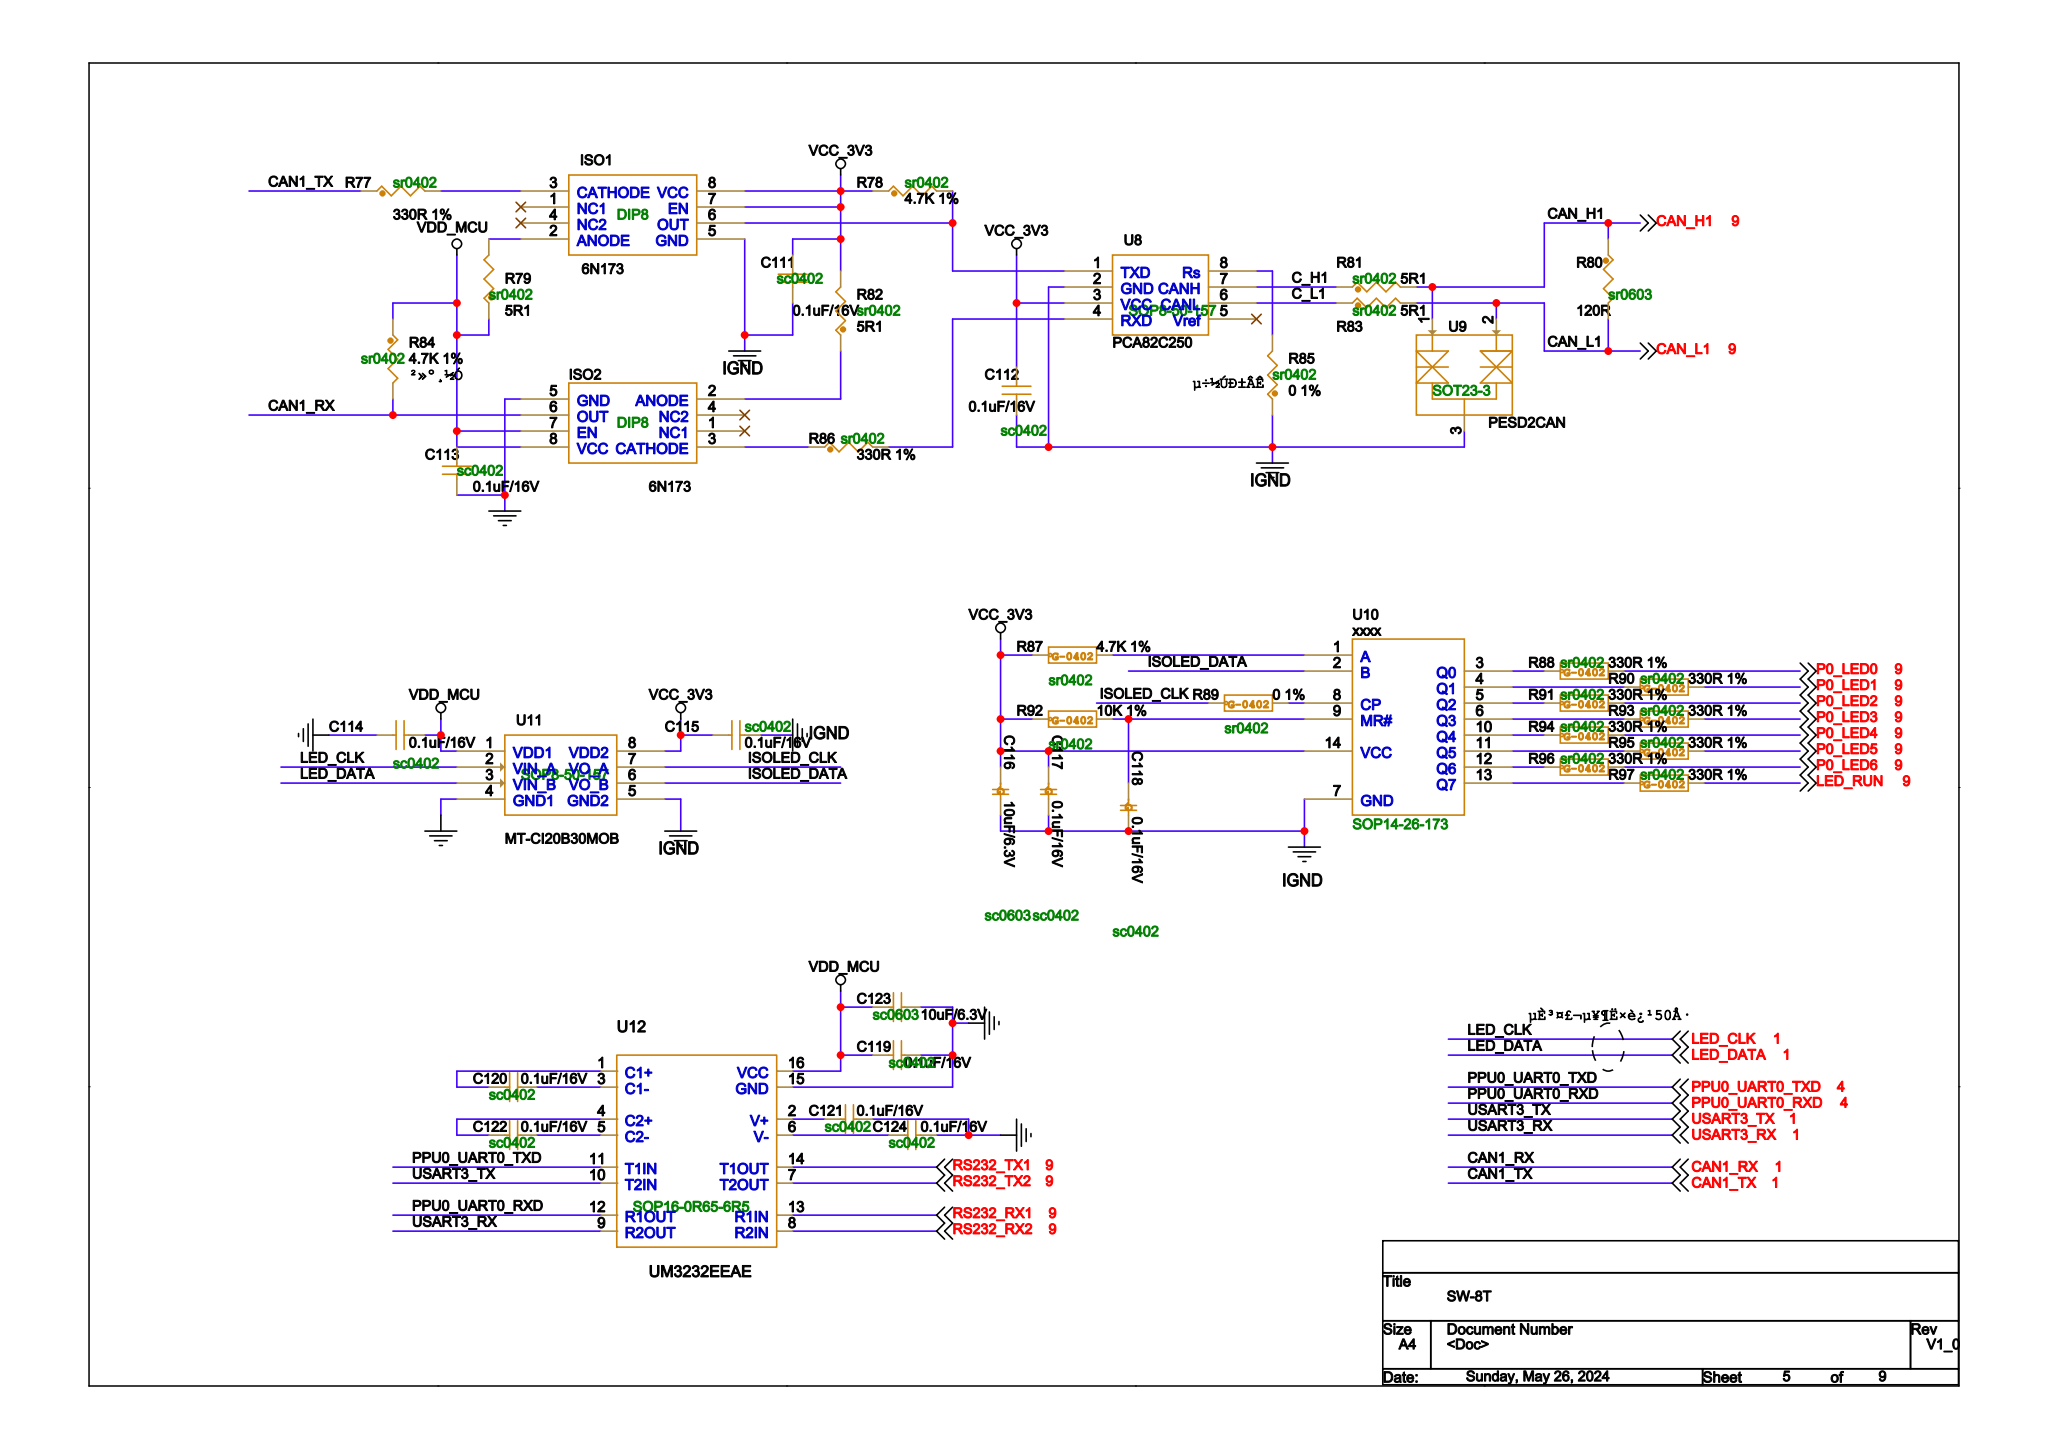Circuit board | Cadence Allegro | 399 parts | 387 nets | one sheet of the schematic
Parts on this sheet (reference | value | footprint):
C111 | 0.1uF/16V | SC0402
C112 | 0.1uF/16V | SC0402
C113 | 0.1uF/16V | SC0402
C114 | 0.1uF/16V | SC0402
C115 | 0.1uF/16V | SC0402
C116 | 10uF/6.3V | SC0603
C117 | 0.1uF/16V | SC0402
C118 | 0.1uF/16V | SC0402
C119 | 0.1uF/16V | SC0402
C120 | 0.1uF/16V | SC0402
C121 | 0.1uF/16V | SC0402
C122 | 0.1uF/16V | SC0402
C123 | 10uF/6.3V | SC0603
C124 | 0.1uF/16V | SC0402
ISO1 | 6N173 | DIP8
ISO2 | 6N173 | DIP8
R77 | 330R 1% | SR0402
R78 | 4.7K 1% | SR0402
R79 | 5R1 | SR0402
R80 | 120R | SR0603
R81 | 5R1 | SR0402
R82 | 5R1 | SR0402
R83 | 5R1 | SR0402
R84 | 4.7K 1% | SR0402
R85 | 0 1% | SR0402
R86 | 330R 1% | SR0402
R87 | 4.7K 1% | SR0402
R88 | 330R 1% | SR0402
R89 | 0 1% | SR0402
R90 | 330R 1% | SR0402
R91 | 330R 1% | SR0402
R92 | 10K 1% | SR0402
R93 | 330R 1% | SR0402
R94 | 330R 1% | SR0402
R95 | 330R 1% | SR0402
R96 | 330R 1% | SR0402
R97 | 330R 1% | SR0402
U8 | PCA82C250 | SOP8-50-157
U9 | PESD2CAN | SOT23-3
U10 | xxxx | SOP14-26-173
U11 | MT-CI20B30MOB | SOP8-50-157
U12 | MAX3232E | SOP16-0R65-6R5
Nets of these parts (net: part-pin ...):
N17727171: C120-2 U12-1
N17727107: C120-1 U12-3
N17727156: C122-2 U12-4
N17727109: C122-1 U12-5
GND: C113-2 C114-1 C119-1 C121-1 C123-1 C124-2 ISO2-5 U11-4 U12-15
RS232_RX1: U12-13
PPU0_UART0_RXD: U12-12
RS232_RX2: U12-8
USART3_RX: U12-9
PPU0_UART0_TXD: U12-11
RS232_TX1: U12-14
USART3_TX: U12-10
RS232_TX2: U12-7
N17727154: C121-2 U12-2
N17727186: C124-1 U12-6
VDD_MCU: C113-1 C114-2 C119-2 C123-2 ISO2-7 ISO2-8 R79-1 R84-1 U11-1 U12-16
VCC_3V3: C111-1 C112-1 C115-1 C116-1 C117-1 ISO1-7 ISO1-8 R78-1 R82-2 R87-1 R92-1 U8-3 U10-14 U11-8
AGND: C111-2 C112-2 C115-2 C116-2 C117-2 C118-2 ISO1-5 R85-1 U8-2 U9-3 U10-7 U11-5
N17745145: C118-1 R92-2 U10-9
N17750169: ISO1-2 R79-2
N17750232: ISO1-3 R77-2
N17750192: ISO1-6 R78-2 U8-1
N17750230: ISO2-2 R82-1
N17750236: ISO2-3 R86-1
CAN1_RX: ISO2-6 R84-2
P0_LED0: R88-2
P0_LED4: R94-2
P0_LED1: R90-2
P0_LED5: R95-2
CAN_L1: R80-2 R83-2 U9-2
CAN_H1: R80-1 R81-2 U9-1
P0_LED6: R96-2
LED_RUN: R97-2
P0_LED2: R91-2
P0_LED3: R93-2
ISOLED_CLK: R89-1 U11-7
N17745328: R89-2 U10-8
N17745148: R87-2 U10-1
CAN1_TX: R77-1
N17750266: R86-2 U8-4
C_H1: R81-1 U8-7
C_L1: R83-1 U8-6
N17750965: R85-2 U8-8
N17745325: R88-1 U10-3
N17745076: R90-1 U10-4
N17745079: R91-1 U10-5
N17745082: R93-1 U10-6
N17745093: R94-1 U10-10
N17745096: R95-1 U10-11
N17745107: R96-1 U10-12
N17745115: R97-1 U10-13
LED_DATA: U11-3
LED_CLK: U11-2
ISOLED_DATA: U10-2 U11-6